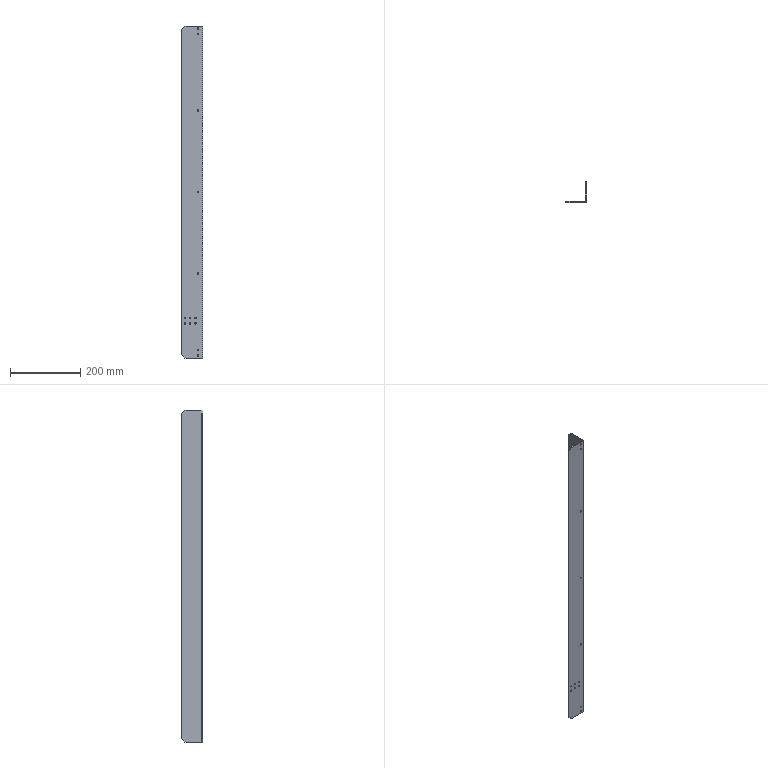Part | SolidWorks | features HoleWzd 2, Chamfer 1, Extrusion 1 | 1 solid | 38 faces | box 60 x 60 x 945 mm | volume 330466 mm3 | cylinder 26 | plane 12 | commonest cylinder face diameters 4.8 x14 4.2 x12
STEP:
#1=CARTESIAN_POINT('',(9.75,0.,-375.8));
#2=VERTEX_POINT('',#1);
#3=CARTESIAN_POINT('',(9.75,0.,-371.6));
#4=VERTEX_POINT('',#3);
#5=CARTESIAN_POINT('',(9.75,0.,-373.7));
#6=DIRECTION('',(0.,1.,0.));
#7=DIRECTION('',(0.,0.,1.));
#8=AXIS2_PLACEMENT_3D('',#5,#6,#7);
#9=CIRCLE('',#8,2.1);
#10=EDGE_CURVE('',#2,#4,#9,.T.);
#11=ORIENTED_EDGE('',*,*,#10,.F.);
#12=CARTESIAN_POINT('',(9.75,3.,-375.8));
#13=VERTEX_POINT('',#12);
#14=CARTESIAN_POINT('',(9.75,3.,-375.8));
#15=DIRECTION('',(0.,1.,0.));
#16=VECTOR('',#15,1000.);
#17=LINE('',#14,#16);
#18=EDGE_CURVE('',#2,#13,#17,.T.);
#19=ORIENTED_EDGE('',*,*,#18,.T.);
#20=CARTESIAN_POINT('',(9.75,3.,-371.6));
#21=VERTEX_POINT('',#20);
#22=CARTESIAN_POINT('',(9.75,3.,-373.7));
#23=DIRECTION('',(0.,1.,0.));
#24=DIRECTION('',(0.,0.,1.));
#25=AXIS2_PLACEMENT_3D('',#22,#23,#24);
#26=CIRCLE('',#25,2.1);
#27=EDGE_CURVE('',#13,#21,#26,.T.);
#28=ORIENTED_EDGE('',*,*,#27,.T.);
#29=CARTESIAN_POINT('',(9.75,3.,-371.6));
#30=DIRECTION('',(0.,1.,0.));
#31=VECTOR('',#30,1000.);
#32=LINE('',#29,#31);
#33=EDGE_CURVE('',#4,#21,#32,.T.);
#34=ORIENTED_EDGE('',*,*,#33,.F.);
#35=EDGE_LOOP('',(#11,#19,#28,#34));
#36=FACE_OUTER_BOUND('',#35,.T.);
#37=CARTESIAN_POINT('',(9.75,3.,-373.7));
#38=DIRECTION('',(0.,1.,0.));
#39=DIRECTION('',(0.,0.,1.));
#40=AXIS2_PLACEMENT_3D('',#37,#38,#39);
#41=CYLINDRICAL_SURFACE('',#40,2.1);
#42=ADVANCED_FACE('',(#36),#41,.F.);
#43=CARTESIAN_POINT('',(39.75,0.,-375.8));
#44=VERTEX_POINT('',#43);
#45=CARTESIAN_POINT('',(39.75,0.,-371.6));
#46=VERTEX_POINT('',#45);
#47=CARTESIAN_POINT('',(39.75,0.,-373.7));
#48=DIRECTION('',(0.,1.,0.));
#49=DIRECTION('',(0.,0.,1.));
#50=AXIS2_PLACEMENT_3D('',#47,#48,#49);
#51=CIRCLE('',#50,2.1);
#52=EDGE_CURVE('',#44,#46,#51,.T.);
#53=ORIENTED_EDGE('',*,*,#52,.F.);
#54=CARTESIAN_POINT('',(39.75,3.,-375.8));
#55=VERTEX_POINT('',#54);
#56=CARTESIAN_POINT('',(39.75,3.,-375.8));
#57=DIRECTION('',(0.,1.,0.));
#58=VECTOR('',#57,1000.);
#59=LINE('',#56,#58);
#60=EDGE_CURVE('',#44,#55,#59,.T.);
#61=ORIENTED_EDGE('',*,*,#60,.T.);
#62=CARTESIAN_POINT('',(39.75,3.,-371.6));
#63=VERTEX_POINT('',#62);
#64=CARTESIAN_POINT('',(39.75,3.,-373.7));
#65=DIRECTION('',(0.,1.,0.));
#66=DIRECTION('',(0.,0.,1.));
#67=AXIS2_PLACEMENT_3D('',#64,#65,#66);
#68=CIRCLE('',#67,2.1);
#69=EDGE_CURVE('',#55,#63,#68,.T.);
#70=ORIENTED_EDGE('',*,*,#69,.T.);
#71=CARTESIAN_POINT('',(39.75,3.,-371.6));
#72=DIRECTION('',(0.,1.,0.));
#73=VECTOR('',#72,1000.);
#74=LINE('',#71,#73);
#75=EDGE_CURVE('',#46,#63,#74,.T.);
#76=ORIENTED_EDGE('',*,*,#75,.F.);
#77=EDGE_LOOP('',(#53,#61,#70,#76));
#78=FACE_OUTER_BOUND('',#77,.T.);
#79=CARTESIAN_POINT('',(39.75,3.,-373.7));
#80=DIRECTION('',(0.,1.,0.));
#81=DIRECTION('',(0.,0.,1.));
#82=AXIS2_PLACEMENT_3D('',#79,#80,#81);
#83=CYLINDRICAL_SURFACE('',#82,2.1);
#84=ADVANCED_FACE('',(#78),#83,.F.);
#85=CARTESIAN_POINT('',(24.75,0.,-360.8));
#86=VERTEX_POINT('',#85);
#87=CARTESIAN_POINT('',(24.75,0.,-356.6));
#88=VERTEX_POINT('',#87);
#89=CARTESIAN_POINT('',(24.75,0.,-358.7));
#90=DIRECTION('',(0.,1.,0.));
#91=DIRECTION('',(0.,0.,1.));
#92=AXIS2_PLACEMENT_3D('',#89,#90,#91);
#93=CIRCLE('',#92,2.1);
#94=EDGE_CURVE('',#86,#88,#93,.T.);
#95=ORIENTED_EDGE('',*,*,#94,.F.);
#96=CARTESIAN_POINT('',(24.75,3.,-360.8));
#97=VERTEX_POINT('',#96);
#98=CARTESIAN_POINT('',(24.75,3.,-360.8));
#99=DIRECTION('',(0.,1.,0.));
#100=VECTOR('',#99,1000.);
#101=LINE('',#98,#100);
#102=EDGE_CURVE('',#86,#97,#101,.T.);
#103=ORIENTED_EDGE('',*,*,#102,.T.);
#104=CARTESIAN_POINT('',(24.75,3.,-356.6));
#105=VERTEX_POINT('',#104);
#106=CARTESIAN_POINT('',(24.75,3.,-358.7));
#107=DIRECTION('',(0.,1.,0.));
#108=DIRECTION('',(0.,0.,1.));
#109=AXIS2_PLACEMENT_3D('',#106,#107,#108);
#110=CIRCLE('',#109,2.1);
#111=EDGE_CURVE('',#97,#105,#110,.T.);
#112=ORIENTED_EDGE('',*,*,#111,.T.);
#113=CARTESIAN_POINT('',(24.75,3.,-356.6));
#114=DIRECTION('',(0.,1.,0.));
#115=VECTOR('',#114,1000.);
#116=LINE('',#113,#115);
#117=EDGE_CURVE('',#88,#105,#116,.T.);
#118=ORIENTED_EDGE('',*,*,#117,.F.);
#119=EDGE_LOOP('',(#95,#103,#112,#118));
#120=FACE_OUTER_BOUND('',#119,.T.);
#121=CARTESIAN_POINT('',(24.75,3.,-358.7));
#122=DIRECTION('',(0.,1.,0.));
#123=DIRECTION('',(0.,0.,1.));
#124=AXIS2_PLACEMENT_3D('',#121,#122,#123);
#125=CYLINDRICAL_SURFACE('',#124,2.1);
#126=ADVANCED_FACE('',(#120),#125,.F.);
#127=CARTESIAN_POINT('',(9.75,0.,-360.8));
#128=VERTEX_POINT('',#127);
#129=CARTESIAN_POINT('',(9.75,0.,-356.6));
#130=VERTEX_POINT('',#129);
#131=CARTESIAN_POINT('',(9.75,0.,-358.7));
#132=DIRECTION('',(0.,1.,0.));
#133=DIRECTION('',(0.,0.,1.));
#134=AXIS2_PLACEMENT_3D('',#131,#132,#133);
#135=CIRCLE('',#134,2.1);
#136=EDGE_CURVE('',#128,#130,#135,.T.);
#137=ORIENTED_EDGE('',*,*,#136,.F.);
#138=CARTESIAN_POINT('',(9.75,3.,-360.8));
#139=VERTEX_POINT('',#138);
#140=CARTESIAN_POINT('',(9.75,3.,-360.8));
#141=DIRECTION('',(0.,1.,0.));
#142=VECTOR('',#141,1000.);
#143=LINE('',#140,#142);
#144=EDGE_CURVE('',#128,#139,#143,.T.);
#145=ORIENTED_EDGE('',*,*,#144,.T.);
#146=CARTESIAN_POINT('',(9.75,3.,-356.6));
#147=VERTEX_POINT('',#146);
#148=CARTESIAN_POINT('',(9.75,3.,-358.7));
#149=DIRECTION('',(0.,1.,0.));
#150=DIRECTION('',(0.,0.,1.));
#151=AXIS2_PLACEMENT_3D('',#148,#149,#150);
#152=CIRCLE('',#151,2.1);
#153=EDGE_CURVE('',#139,#147,#152,.T.);
#154=ORIENTED_EDGE('',*,*,#153,.T.);
#155=CARTESIAN_POINT('',(9.75,3.,-356.6));
#156=DIRECTION('',(0.,1.,0.));
#157=VECTOR('',#156,1000.);
#158=LINE('',#155,#157);
#159=EDGE_CURVE('',#130,#147,#158,.T.);
#160=ORIENTED_EDGE('',*,*,#159,.F.);
#161=EDGE_LOOP('',(#137,#145,#154,#160));
#162=FACE_OUTER_BOUND('',#161,.T.);
#163=CARTESIAN_POINT('',(9.75,3.,-358.7));
#164=DIRECTION('',(0.,1.,0.));
#165=DIRECTION('',(0.,0.,1.));
#166=AXIS2_PLACEMENT_3D('',#163,#164,#165);
#167=CYLINDRICAL_SURFACE('',#166,2.1);
#168=ADVANCED_FACE('',(#162),#167,.F.);
#169=CARTESIAN_POINT('',(39.75,0.,-360.8));
#170=VERTEX_POINT('',#169);
#171=CARTESIAN_POINT('',(39.75,0.,-356.6));
#172=VERTEX_POINT('',#171);
#173=CARTESIAN_POINT('',(39.75,0.,-358.7));
#174=DIRECTION('',(0.,1.,0.));
#175=DIRECTION('',(0.,0.,1.));
#176=AXIS2_PLACEMENT_3D('',#173,#174,#175);
#177=CIRCLE('',#176,2.1);
#178=EDGE_CURVE('',#170,#172,#177,.T.);
#179=ORIENTED_EDGE('',*,*,#178,.F.);
#180=CARTESIAN_POINT('',(39.75,3.,-360.8));
#181=VERTEX_POINT('',#180);
#182=CARTESIAN_POINT('',(39.75,3.,-360.8));
#183=DIRECTION('',(0.,1.,0.));
#184=VECTOR('',#183,1000.);
#185=LINE('',#182,#184);
#186=EDGE_CURVE('',#170,#181,#185,.T.);
#187=ORIENTED_EDGE('',*,*,#186,.T.);
#188=CARTESIAN_POINT('',(39.75,3.,-356.6));
#189=VERTEX_POINT('',#188);
#190=CARTESIAN_POINT('',(39.75,3.,-358.7));
#191=DIRECTION('',(0.,1.,0.));
#192=DIRECTION('',(0.,0.,1.));
#193=AXIS2_PLACEMENT_3D('',#190,#191,#192);
#194=CIRCLE('',#193,2.1);
#195=EDGE_CURVE('',#181,#189,#194,.T.);
#196=ORIENTED_EDGE('',*,*,#195,.T.);
#197=CARTESIAN_POINT('',(39.75,3.,-356.6));
#198=DIRECTION('',(0.,1.,0.));
#199=VECTOR('',#198,1000.);
#200=LINE('',#197,#199);
#201=EDGE_CURVE('',#172,#189,#200,.T.);
#202=ORIENTED_EDGE('',*,*,#201,.F.);
#203=EDGE_LOOP('',(#179,#187,#196,#202));
#204=FACE_OUTER_BOUND('',#203,.T.);
#205=CARTESIAN_POINT('',(39.75,3.,-358.7));
#206=DIRECTION('',(0.,1.,0.));
#207=DIRECTION('',(0.,0.,1.));
#208=AXIS2_PLACEMENT_3D('',#205,#206,#207);
#209=CYLINDRICAL_SURFACE('',#208,2.1);
#210=ADVANCED_FACE('',(#204),#209,.F.);
#211=CARTESIAN_POINT('',(24.75,0.,-375.8));
#212=VERTEX_POINT('',#211);
#213=CARTESIAN_POINT('',(24.75,0.,-371.6));
#214=VERTEX_POINT('',#213);
#215=CARTESIAN_POINT('',(24.75,0.,-373.7));
#216=DIRECTION('',(0.,1.,0.));
#217=DIRECTION('',(0.,0.,1.));
#218=AXIS2_PLACEMENT_3D('',#215,#216,#217);
#219=CIRCLE('',#218,2.1);
#220=EDGE_CURVE('',#212,#214,#219,.T.);
#221=ORIENTED_EDGE('',*,*,#220,.F.);
#222=CARTESIAN_POINT('',(24.75,3.,-375.8));
#223=VERTEX_POINT('',#222);
#224=CARTESIAN_POINT('',(24.75,3.,-375.8));
#225=DIRECTION('',(0.,1.,0.));
#226=VECTOR('',#225,1000.);
#227=LINE('',#224,#226);
#228=EDGE_CURVE('',#212,#223,#227,.T.);
#229=ORIENTED_EDGE('',*,*,#228,.T.);
#230=CARTESIAN_POINT('',(24.75,3.,-371.6));
#231=VERTEX_POINT('',#230);
#232=CARTESIAN_POINT('',(24.75,3.,-373.7));
#233=DIRECTION('',(0.,1.,0.));
#234=DIRECTION('',(0.,0.,1.));
#235=AXIS2_PLACEMENT_3D('',#232,#233,#234);
#236=CIRCLE('',#235,2.1);
#237=EDGE_CURVE('',#223,#231,#236,.T.);
#238=ORIENTED_EDGE('',*,*,#237,.T.);
#239=CARTESIAN_POINT('',(24.75,3.,-371.6));
#240=DIRECTION('',(0.,1.,0.));
#241=VECTOR('',#240,1000.);
#242=LINE('',#239,#241);
#243=EDGE_CURVE('',#214,#231,#242,.T.);
#244=ORIENTED_EDGE('',*,*,#243,.F.);
#245=EDGE_LOOP('',(#221,#229,#238,#244));
#246=FACE_OUTER_BOUND('',#245,.T.);
#247=CARTESIAN_POINT('',(24.75,3.,-373.7));
#248=DIRECTION('',(0.,1.,0.));
#249=DIRECTION('',(0.,0.,1.));
#250=AXIS2_PLACEMENT_3D('',#247,#248,#249);
#251=CYLINDRICAL_SURFACE('',#250,2.1);
#252=ADVANCED_FACE('',(#246),#251,.F.);
#253=CARTESIAN_POINT('',(47.,0.,-2.4));
#254=VERTEX_POINT('',#253);
#255=CARTESIAN_POINT('',(47.,0.,2.4));
#256=VERTEX_POINT('',#255);
#257=CARTESIAN_POINT('',(47.,0.,0.));
#258=DIRECTION('',(0.,1.,0.));
#259=DIRECTION('',(0.,0.,1.));
#260=AXIS2_PLACEMENT_3D('',#257,#258,#259);
#261=CIRCLE('',#260,2.4);
#262=EDGE_CURVE('',#254,#256,#261,.T.);
#263=ORIENTED_EDGE('',*,*,#262,.F.);
#264=CARTESIAN_POINT('',(47.,3.,-2.4));
#265=VERTEX_POINT('',#264);
#266=CARTESIAN_POINT('',(47.,3.,-2.4));
#267=DIRECTION('',(0.,1.,0.));
#268=VECTOR('',#267,1000.);
#269=LINE('',#266,#268);
#270=EDGE_CURVE('',#254,#265,#269,.T.);
#271=ORIENTED_EDGE('',*,*,#270,.T.);
#272=CARTESIAN_POINT('',(47.,3.,2.4));
#273=VERTEX_POINT('',#272);
#274=CARTESIAN_POINT('',(47.,3.,0.));
#275=DIRECTION('',(0.,1.,0.));
#276=DIRECTION('',(0.,0.,1.));
#277=AXIS2_PLACEMENT_3D('',#274,#275,#276);
#278=CIRCLE('',#277,2.4);
#279=EDGE_CURVE('',#265,#273,#278,.T.);
#280=ORIENTED_EDGE('',*,*,#279,.T.);
#281=CARTESIAN_POINT('',(47.,3.,2.4));
#282=DIRECTION('',(0.,1.,0.));
#283=VECTOR('',#282,1000.);
#284=LINE('',#281,#283);
#285=EDGE_CURVE('',#256,#273,#284,.T.);
#286=ORIENTED_EDGE('',*,*,#285,.F.);
#287=EDGE_LOOP('',(#263,#271,#280,#286));
#288=FACE_OUTER_BOUND('',#287,.T.);
#289=CARTESIAN_POINT('',(47.,3.,0.));
#290=DIRECTION('',(0.,1.,0.));
#291=DIRECTION('',(0.,0.,1.));
#292=AXIS2_PLACEMENT_3D('',#289,#290,#291);
#293=CYLINDRICAL_SURFACE('',#292,2.4);
#294=ADVANCED_FACE('',(#288),#293,.F.);
#295=CARTESIAN_POINT('',(47.,0.,-234.65));
#296=VERTEX_POINT('',#295);
#297=CARTESIAN_POINT('',(47.,0.,-229.85));
#298=VERTEX_POINT('',#297);
#299=CARTESIAN_POINT('',(47.,0.,-232.25));
#300=DIRECTION('',(0.,1.,0.));
#301=DIRECTION('',(0.,0.,1.));
#302=AXIS2_PLACEMENT_3D('',#299,#300,#301);
#303=CIRCLE('',#302,2.4);
#304=EDGE_CURVE('',#296,#298,#303,.T.);
#305=ORIENTED_EDGE('',*,*,#304,.F.);
#306=CARTESIAN_POINT('',(47.,3.,-234.65));
#307=VERTEX_POINT('',#306);
#308=CARTESIAN_POINT('',(47.,3.,-234.65));
#309=DIRECTION('',(0.,1.,0.));
#310=VECTOR('',#309,1000.);
#311=LINE('',#308,#310);
#312=EDGE_CURVE('',#296,#307,#311,.T.);
#313=ORIENTED_EDGE('',*,*,#312,.T.);
#314=CARTESIAN_POINT('',(47.,3.,-229.85));
#315=VERTEX_POINT('',#314);
#316=CARTESIAN_POINT('',(47.,3.,-232.25));
#317=DIRECTION('',(0.,1.,0.));
#318=DIRECTION('',(0.,0.,1.));
#319=AXIS2_PLACEMENT_3D('',#316,#317,#318);
#320=CIRCLE('',#319,2.4);
#321=EDGE_CURVE('',#307,#315,#320,.T.);
#322=ORIENTED_EDGE('',*,*,#321,.T.);
#323=CARTESIAN_POINT('',(47.,3.,-229.85));
#324=DIRECTION('',(0.,1.,0.));
#325=VECTOR('',#324,1000.);
#326=LINE('',#323,#325);
#327=EDGE_CURVE('',#298,#315,#326,.T.);
#328=ORIENTED_EDGE('',*,*,#327,.F.);
#329=EDGE_LOOP('',(#305,#313,#322,#328));
#330=FACE_OUTER_BOUND('',#329,.T.);
#331=CARTESIAN_POINT('',(47.,3.,-232.25));
#332=DIRECTION('',(0.,1.,0.));
#333=DIRECTION('',(0.,0.,1.));
#334=AXIS2_PLACEMENT_3D('',#331,#332,#333);
#335=CYLINDRICAL_SURFACE('',#334,2.4);
#336=ADVANCED_FACE('',(#330),#335,.F.);
#337=CARTESIAN_POINT('',(47.,0.,-466.9));
#338=VERTEX_POINT('',#337);
#339=CARTESIAN_POINT('',(47.,0.,-462.1));
#340=VERTEX_POINT('',#339);
#341=CARTESIAN_POINT('',(47.,0.,-464.5));
#342=DIRECTION('',(0.,1.,0.));
#343=DIRECTION('',(0.,0.,1.));
#344=AXIS2_PLACEMENT_3D('',#341,#342,#343);
#345=CIRCLE('',#344,2.4);
#346=EDGE_CURVE('',#338,#340,#345,.T.);
#347=ORIENTED_EDGE('',*,*,#346,.F.);
#348=CARTESIAN_POINT('',(47.,3.,-466.9));
#349=VERTEX_POINT('',#348);
#350=CARTESIAN_POINT('',(47.,3.,-466.9));
#351=DIRECTION('',(0.,1.,0.));
#352=VECTOR('',#351,1000.);
#353=LINE('',#350,#352);
#354=EDGE_CURVE('',#338,#349,#353,.T.);
#355=ORIENTED_EDGE('',*,*,#354,.T.);
#356=CARTESIAN_POINT('',(47.,3.,-462.1));
#357=VERTEX_POINT('',#356);
#358=CARTESIAN_POINT('',(47.,3.,-464.5));
#359=DIRECTION('',(0.,1.,0.));
#360=DIRECTION('',(0.,0.,1.));
#361=AXIS2_PLACEMENT_3D('',#358,#359,#360);
#362=CIRCLE('',#361,2.4);
#363=EDGE_CURVE('',#349,#357,#362,.T.);
#364=ORIENTED_EDGE('',*,*,#363,.T.);
#365=CARTESIAN_POINT('',(47.,3.,-462.1));
#366=DIRECTION('',(0.,1.,0.));
#367=VECTOR('',#366,1000.);
#368=LINE('',#365,#367);
#369=EDGE_CURVE('',#340,#357,#368,.T.);
#370=ORIENTED_EDGE('',*,*,#369,.F.);
#371=EDGE_LOOP('',(#347,#355,#364,#370));
#372=FACE_OUTER_BOUND('',#371,.T.);
#373=CARTESIAN_POINT('',(47.,3.,-464.5));
#374=DIRECTION('',(0.,1.,0.));
#375=DIRECTION('',(0.,0.,1.));
#376=AXIS2_PLACEMENT_3D('',#373,#374,#375);
#377=CYLINDRICAL_SURFACE('',#376,2.4);
#378=ADVANCED_FACE('',(#372),#377,.F.);
#379=CARTESIAN_POINT('',(47.,0.,462.1));
#380=VERTEX_POINT('',#379);
#381=CARTESIAN_POINT('',(47.,0.,466.9));
#382=VERTEX_POINT('',#381);
#383=CARTESIAN_POINT('',(47.,0.,464.5));
#384=DIRECTION('',(0.,1.,0.));
#385=DIRECTION('',(0.,0.,1.));
#386=AXIS2_PLACEMENT_3D('',#383,#384,#385);
#387=CIRCLE('',#386,2.4);
#388=EDGE_CURVE('',#380,#382,#387,.T.);
#389=ORIENTED_EDGE('',*,*,#388,.F.);
#390=CARTESIAN_POINT('',(47.,3.,462.1));
#391=VERTEX_POINT('',#390);
#392=CARTESIAN_POINT('',(47.,3.,462.1));
#393=DIRECTION('',(0.,1.,0.));
#394=VECTOR('',#393,1000.);
#395=LINE('',#392,#394);
#396=EDGE_CURVE('',#380,#391,#395,.T.);
#397=ORIENTED_EDGE('',*,*,#396,.T.);
#398=CARTESIAN_POINT('',(47.,3.,466.9));
#399=VERTEX_POINT('',#398);
#400=CARTESIAN_POINT('',(47.,3.,464.5));
#401=DIRECTION('',(0.,1.,0.));
#402=DIRECTION('',(0.,0.,1.));
#403=AXIS2_PLACEMENT_3D('',#400,#401,#402);
#404=CIRCLE('',#403,2.4);
#405=EDGE_CURVE('',#391,#399,#404,.T.);
#406=ORIENTED_EDGE('',*,*,#405,.T.);
#407=CARTESIAN_POINT('',(47.,3.,466.9));
#408=DIRECTION('',(0.,1.,0.));
#409=VECTOR('',#408,1000.);
#410=LINE('',#407,#409);
#411=EDGE_CURVE('',#382,#399,#410,.T.);
#412=ORIENTED_EDGE('',*,*,#411,.F.);
#413=EDGE_LOOP('',(#389,#397,#406,#412));
#414=FACE_OUTER_BOUND('',#413,.T.);
#415=CARTESIAN_POINT('',(47.,3.,464.5));
#416=DIRECTION('',(0.,1.,0.));
#417=DIRECTION('',(0.,0.,1.));
#418=AXIS2_PLACEMENT_3D('',#415,#416,#417);
#419=CYLINDRICAL_SURFACE('',#418,2.4);
#420=ADVANCED_FACE('',(#414),#419,.F.);
#421=CARTESIAN_POINT('',(47.,0.,229.85));
#422=VERTEX_POINT('',#421);
#423=CARTESIAN_POINT('',(47.,0.,234.65));
#424=VERTEX_POINT('',#423);
#425=CARTESIAN_POINT('',(47.,0.,232.25));
#426=DIRECTION('',(0.,1.,0.));
#427=DIRECTION('',(0.,0.,1.));
#428=AXIS2_PLACEMENT_3D('',#425,#426,#427);
#429=CIRCLE('',#428,2.4);
#430=EDGE_CURVE('',#422,#424,#429,.T.);
#431=ORIENTED_EDGE('',*,*,#430,.F.);
#432=CARTESIAN_POINT('',(47.,3.,229.85));
#433=VERTEX_POINT('',#432);
#434=CARTESIAN_POINT('',(47.,3.,229.85));
#435=DIRECTION('',(0.,1.,0.));
#436=VECTOR('',#435,1000.);
#437=LINE('',#434,#436);
#438=EDGE_CURVE('',#422,#433,#437,.T.);
#439=ORIENTED_EDGE('',*,*,#438,.T.);
#440=CARTESIAN_POINT('',(47.,3.,234.65));
#441=VERTEX_POINT('',#440);
#442=CARTESIAN_POINT('',(47.,3.,232.25));
#443=DIRECTION('',(0.,1.,0.));
#444=DIRECTION('',(0.,0.,1.));
#445=AXIS2_PLACEMENT_3D('',#442,#443,#444);
#446=CIRCLE('',#445,2.4);
#447=EDGE_CURVE('',#433,#441,#446,.T.);
#448=ORIENTED_EDGE('',*,*,#447,.T.);
#449=CARTESIAN_POINT('',(47.,3.,234.65));
#450=DIRECTION('',(0.,1.,0.));
#451=VECTOR('',#450,1000.);
#452=LINE('',#449,#451);
#453=EDGE_CURVE('',#424,#441,#452,.T.);
#454=ORIENTED_EDGE('',*,*,#453,.F.);
#455=EDGE_LOOP('',(#431,#439,#448,#454));
#456=FACE_OUTER_BOUND('',#455,.T.);
#457=CARTESIAN_POINT('',(47.,3.,232.25));
#458=DIRECTION('',(0.,1.,0.));
#459=DIRECTION('',(0.,0.,1.));
#460=AXIS2_PLACEMENT_3D('',#457,#458,#459);
#461=CYLINDRICAL_SURFACE('',#460,2.4);
#462=ADVANCED_FACE('',(#456),#461,.F.);
#463=CARTESIAN_POINT('',(47.,0.,-451.9));
#464=VERTEX_POINT('',#463);
#465=CARTESIAN_POINT('',(47.,0.,-447.1));
#466=VERTEX_POINT('',#465);
#467=CARTESIAN_POINT('',(47.,0.,-449.5));
#468=DIRECTION('',(0.,1.,0.));
#469=DIRECTION('',(0.,0.,1.));
#470=AXIS2_PLACEMENT_3D('',#467,#468,#469);
#471=CIRCLE('',#470,2.4);
#472=EDGE_CURVE('',#464,#466,#471,.T.);
#473=ORIENTED_EDGE('',*,*,#472,.F.);
#474=CARTESIAN_POINT('',(47.,3.,-451.9));
#475=VERTEX_POINT('',#474);
#476=CARTESIAN_POINT('',(47.,3.,-451.9));
#477=DIRECTION('',(0.,1.,0.));
#478=VECTOR('',#477,1000.);
#479=LINE('',#476,#478);
#480=EDGE_CURVE('',#464,#475,#479,.T.);
#481=ORIENTED_EDGE('',*,*,#480,.T.);
#482=CARTESIAN_POINT('',(47.,3.,-447.1));
#483=VERTEX_POINT('',#482);
#484=CARTESIAN_POINT('',(47.,3.,-449.5));
#485=DIRECTION('',(0.,1.,0.));
#486=DIRECTION('',(0.,0.,1.));
#487=AXIS2_PLACEMENT_3D('',#484,#485,#486);
#488=CIRCLE('',#487,2.4);
#489=EDGE_CURVE('',#475,#483,#488,.T.);
#490=ORIENTED_EDGE('',*,*,#489,.T.);
#491=CARTESIAN_POINT('',(47.,3.,-447.1));
#492=DIRECTION('',(0.,1.,0.));
#493=VECTOR('',#492,1000.);
#494=LINE('',#491,#493);
#495=EDGE_CURVE('',#466,#483,#494,.T.);
#496=ORIENTED_EDGE('',*,*,#495,.F.);
#497=EDGE_LOOP('',(#473,#481,#490,#496));
#498=FACE_OUTER_BOUND('',#497,.T.);
#499=CARTESIAN_POINT('',(47.,3.,-449.5));
#500=DIRECTION('',(0.,1.,0.));
#501=DIRECTION('',(0.,0.,1.));
#502=AXIS2_PLACEMENT_3D('',#499,#500,#501);
#503=CYLINDRICAL_SURFACE('',#502,2.4);
#504=ADVANCED_FACE('',(#498),#503,.F.);
#505=CARTESIAN_POINT('',(47.,0.,447.1));
#506=VERTEX_POINT('',#505);
#507=CARTESIAN_POINT('',(47.,0.,451.9));
#508=VERTEX_POINT('',#507);
#509=CARTESIAN_POINT('',(47.,0.,449.5));
#510=DIRECTION('',(0.,1.,0.));
#511=DIRECTION('',(0.,0.,1.));
#512=AXIS2_PLACEMENT_3D('',#509,#510,#511);
#513=CIRCLE('',#512,2.4);
#514=EDGE_CURVE('',#506,#508,#513,.T.);
#515=ORIENTED_EDGE('',*,*,#514,.F.);
#516=CARTESIAN_POINT('',(47.,3.,447.1));
#517=VERTEX_POINT('',#516);
#518=CARTESIAN_POINT('',(47.,3.,447.1));
#519=DIRECTION('',(0.,1.,0.));
#520=VECTOR('',#519,1000.);
#521=LINE('',#518,#520);
#522=EDGE_CURVE('',#506,#517,#521,.T.);
#523=ORIENTED_EDGE('',*,*,#522,.T.);
#524=CARTESIAN_POINT('',(47.,3.,451.9));
#525=VERTEX_POINT('',#524);
#526=CARTESIAN_POINT('',(47.,3.,449.5));
#527=DIRECTION('',(0.,1.,0.));
#528=DIRECTION('',(0.,0.,1.));
#529=AXIS2_PLACEMENT_3D('',#526,#527,#528);
#530=CIRCLE('',#529,2.4);
#531=EDGE_CURVE('',#517,#525,#530,.T.);
#532=ORIENTED_EDGE('',*,*,#531,.T.);
#533=CARTESIAN_POINT('',(47.,3.,451.9));
#534=DIRECTION('',(0.,1.,0.));
#535=VECTOR('',#534,1000.);
#536=LINE('',#533,#535);
#537=EDGE_CURVE('',#508,#525,#536,.T.);
#538=ORIENTED_EDGE('',*,*,#537,.F.);
#539=EDGE_LOOP('',(#515,#523,#532,#538));
#540=FACE_OUTER_BOUND('',#539,.T.);
#541=CARTESIAN_POINT('',(47.,3.,449.5));
#542=DIRECTION('',(0.,1.,0.));
#543=DIRECTION('',(0.,0.,1.));
#544=AXIS2_PLACEMENT_3D('',#541,#542,#543);
#545=CYLINDRICAL_SURFACE('',#544,2.4);
#546=ADVANCED_FACE('',(#540),#545,.F.);
#547=CARTESIAN_POINT('',(47.,3.,0.));
#548=DIRECTION('',(0.,1.,0.));
#549=DIRECTION('',(0.,0.,1.));
#550=AXIS2_PLACEMENT_3D('',#547,#548,#549);
#551=CIRCLE('',#550,2.4);
#552=EDGE_CURVE('',#273,#265,#551,.T.);
#553=ORIENTED_EDGE('',*,*,#552,.F.);
#554=ORIENTED_EDGE('',*,*,#279,.F.);
#555=EDGE_LOOP('',(#553,#554));
#556=FACE_BOUND('',#555,.T.);
#557=CARTESIAN_POINT('',(47.,3.,-232.25));
#558=DIRECTION('',(0.,1.,0.));
#559=DIRECTION('',(0.,0.,1.));
#560=AXIS2_PLACEMENT_3D('',#557,#558,#559);
#561=CIRCLE('',#560,2.4);
#562=EDGE_CURVE('',#315,#307,#561,.T.);
#563=ORIENTED_EDGE('',*,*,#562,.F.);
#564=ORIENTED_EDGE('',*,*,#321,.F.);
#565=EDGE_LOOP('',(#563,#564));
#566=FACE_BOUND('',#565,.T.);
#567=CARTESIAN_POINT('',(47.,3.,-464.5));
#568=DIRECTION('',(0.,1.,0.));
#569=DIRECTION('',(0.,0.,1.));
#570=AXIS2_PLACEMENT_3D('',#567,#568,#569);
#571=CIRCLE('',#570,2.4);
#572=EDGE_CURVE('',#357,#349,#571,.T.);
#573=ORIENTED_EDGE('',*,*,#572,.F.);
#574=ORIENTED_EDGE('',*,*,#363,.F.);
#575=EDGE_LOOP('',(#573,#574));
#576=FACE_BOUND('',#575,.T.);
#577=CARTESIAN_POINT('',(47.,3.,464.5));
#578=DIRECTION('',(0.,1.,0.));
#579=DIRECTION('',(0.,0.,1.));
#580=AXIS2_PLACEMENT_3D('',#577,#578,#579);
#581=CIRCLE('',#580,2.4);
#582=EDGE_CURVE('',#399,#391,#581,.T.);
#583=ORIENTED_EDGE('',*,*,#582,.F.);
#584=ORIENTED_EDGE('',*,*,#405,.F.);
#585=EDGE_LOOP('',(#583,#584));
#586=FACE_BOUND('',#585,.T.);
#587=CARTESIAN_POINT('',(47.,3.,232.25));
#588=DIRECTION('',(0.,1.,0.));
#589=DIRECTION('',(0.,0.,1.));
#590=AXIS2_PLACEMENT_3D('',#587,#588,#589);
#591=CIRCLE('',#590,2.4);
#592=EDGE_CURVE('',#441,#433,#591,.T.);
#593=ORIENTED_EDGE('',*,*,#592,.F.);
#594=ORIENTED_EDGE('',*,*,#447,.F.);
#595=EDGE_LOOP('',(#593,#594));
#596=FACE_BOUND('',#595,.T.);
#597=CARTESIAN_POINT('',(47.,3.,-449.5));
#598=DIRECTION('',(0.,1.,0.));
#599=DIRECTION('',(0.,0.,1.));
#600=AXIS2_PLACEMENT_3D('',#597,#598,#599);
#601=CIRCLE('',#600,2.4);
#602=EDGE_CURVE('',#483,#475,#601,.T.);
#603=ORIENTED_EDGE('',*,*,#602,.F.);
#604=ORIENTED_EDGE('',*,*,#489,.F.);
#605=EDGE_LOOP('',(#603,#604));
#606=FACE_BOUND('',#605,.T.);
#607=CARTESIAN_POINT('',(47.,3.,449.5));
#608=DIRECTION('',(0.,1.,0.));
#609=DIRECTION('',(0.,0.,1.));
#610=AXIS2_PLACEMENT_3D('',#607,#608,#609);
#611=CIRCLE('',#610,2.4);
#612=EDGE_CURVE('',#525,#517,#611,.T.);
#613=ORIENTED_EDGE('',*,*,#612,.F.);
#614=ORIENTED_EDGE('',*,*,#531,.F.);
#615=EDGE_LOOP('',(#613,#614));
#616=FACE_BOUND('',#615,.T.);
#617=CARTESIAN_POINT('',(57.,3.,-472.5));
#618=VERTEX_POINT('',#617);
#619=CARTESIAN_POINT('',(10.,3.,-472.5));
#620=VERTEX_POINT('',#619);
#621=CARTESIAN_POINT('',(57.,3.,-472.5));
#622=DIRECTION('',(-1.,0.,0.));
#623=VECTOR('',#622,1000.);
#624=LINE('',#621,#623);
#625=EDGE_CURVE('',#618,#620,#624,.T.);
#626=ORIENTED_EDGE('',*,*,#625,.T.);
#627=CARTESIAN_POINT('',(0.,3.,-462.5));
#628=VERTEX_POINT('',#627);
#629=CARTESIAN_POINT('',(0.,3.,-462.5));
#630=DIRECTION('',(-0.7071,0.,0.7071));
#631=VECTOR('',#630,1000.);
#632=LINE('',#629,#631);
#633=EDGE_CURVE('',#620,#628,#632,.T.);
#634=ORIENTED_EDGE('',*,*,#633,.T.);
#635=CARTESIAN_POINT('',(0.,3.,462.5));
#636=VERTEX_POINT('',#635);
#637=CARTESIAN_POINT('',(0.,3.,472.5));
#638=DIRECTION('',(0.,0.,-1.));
#639=VECTOR('',#638,1000.);
#640=LINE('',#637,#639);
#641=EDGE_CURVE('',#636,#628,#640,.T.);
#642=ORIENTED_EDGE('',*,*,#641,.F.);
#643=CARTESIAN_POINT('',(10.,3.,472.5));
#644=VERTEX_POINT('',#643);
#645=CARTESIAN_POINT('',(10.,3.,472.5));
#646=DIRECTION('',(0.7071,0.,0.7071));
#647=VECTOR('',#646,1000.);
#648=LINE('',#645,#647);
#649=EDGE_CURVE('',#636,#644,#648,.T.);
#650=ORIENTED_EDGE('',*,*,#649,.T.);
#651=CARTESIAN_POINT('',(57.,3.,472.5));
#652=VERTEX_POINT('',#651);
#653=CARTESIAN_POINT('',(57.,3.,472.5));
#654=DIRECTION('',(-1.,0.,0.));
#655=VECTOR('',#654,1000.);
#656=LINE('',#653,#655);
#657=EDGE_CURVE('',#652,#644,#656,.T.);
#658=ORIENTED_EDGE('',*,*,#657,.F.);
#659=CARTESIAN_POINT('',(57.,3.,472.5));
#660=DIRECTION('',(0.,0.,-1.));
#661=VECTOR('',#660,1000.);
#662=LINE('',#659,#661);
#663=EDGE_CURVE('',#652,#618,#662,.T.);
#664=ORIENTED_EDGE('',*,*,#663,.T.);
#665=EDGE_LOOP('',(#626,#634,#642,#650,#658,#664));
#666=FACE_OUTER_BOUND('',#665,.T.);
#667=CARTESIAN_POINT('',(24.75,3.,-373.7));
#668=DIRECTION('',(0.,1.,0.));
#669=DIRECTION('',(0.,0.,1.));
#670=AXIS2_PLACEMENT_3D('',#667,#668,#669);
#671=CIRCLE('',#670,2.1);
#672=EDGE_CURVE('',#231,#223,#671,.T.);
#673=ORIENTED_EDGE('',*,*,#672,.F.);
#674=ORIENTED_EDGE('',*,*,#237,.F.);
#675=EDGE_LOOP('',(#673,#674));
#676=FACE_BOUND('',#675,.T.);
#677=CARTESIAN_POINT('',(39.75,3.,-358.7));
#678=DIRECTION('',(0.,1.,0.));
#679=DIRECTION('',(0.,0.,1.));
#680=AXIS2_PLACEMENT_3D('',#677,#678,#679);
#681=CIRCLE('',#680,2.1);
#682=EDGE_CURVE('',#189,#181,#681,.T.);
#683=ORIENTED_EDGE('',*,*,#682,.F.);
#684=ORIENTED_EDGE('',*,*,#195,.F.);
#685=EDGE_LOOP('',(#683,#684));
#686=FACE_BOUND('',#685,.T.);
#687=CARTESIAN_POINT('',(9.75,3.,-358.7));
#688=DIRECTION('',(0.,1.,0.));
#689=DIRECTION('',(0.,0.,1.));
#690=AXIS2_PLACEMENT_3D('',#687,#688,#689);
#691=CIRCLE('',#690,2.1);
#692=EDGE_CURVE('',#147,#139,#691,.T.);
#693=ORIENTED_EDGE('',*,*,#692,.F.);
#694=ORIENTED_EDGE('',*,*,#153,.F.);
#695=EDGE_LOOP('',(#693,#694));
#696=FACE_BOUND('',#695,.T.);
#697=CARTESIAN_POINT('',(24.75,3.,-358.7));
#698=DIRECTION('',(0.,1.,0.));
#699=DIRECTION('',(0.,0.,1.));
#700=AXIS2_PLACEMENT_3D('',#697,#698,#699);
#701=CIRCLE('',#700,2.1);
#702=EDGE_CURVE('',#105,#97,#701,.T.);
#703=ORIENTED_EDGE('',*,*,#702,.F.);
#704=ORIENTED_EDGE('',*,*,#111,.F.);
#705=EDGE_LOOP('',(#703,#704));
#706=FACE_BOUND('',#705,.T.);
#707=CARTESIAN_POINT('',(39.75,3.,-373.7));
#708=DIRECTION('',(0.,1.,0.));
#709=DIRECTION('',(0.,0.,1.));
#710=AXIS2_PLACEMENT_3D('',#707,#708,#709);
#711=CIRCLE('',#710,2.1);
#712=EDGE_CURVE('',#63,#55,#711,.T.);
#713=ORIENTED_EDGE('',*,*,#712,.F.);
#714=ORIENTED_EDGE('',*,*,#69,.F.);
#715=EDGE_LOOP('',(#713,#714));
#716=FACE_BOUND('',#715,.T.);
#717=CARTESIAN_POINT('',(9.75,3.,-373.7));
#718=DIRECTION('',(0.,1.,0.));
#719=DIRECTION('',(0.,0.,1.));
#720=AXIS2_PLACEMENT_3D('',#717,#718,#719);
#721=CIRCLE('',#720,2.1);
#722=EDGE_CURVE('',#21,#13,#721,.T.);
#723=ORIENTED_EDGE('',*,*,#722,.F.);
#724=ORIENTED_EDGE('',*,*,#27,.F.);
#725=EDGE_LOOP('',(#723,#724));
#726=FACE_BOUND('',#725,.T.);
#727=CARTESIAN_POINT('',(57.,3.,472.5));
#728=DIRECTION('',(0.,-1.,0.));
#729=DIRECTION('',(1.,0.,0.));
#730=AXIS2_PLACEMENT_3D('',#727,#728,#729);
#731=PLANE('',#730);
#732=ADVANCED_FACE('',(#556,#566,#576,#586,#596,#606,#616,#666,#676,#686,#696,#706,#716,#726),#731,.F.);
#733=ORIENTED_EDGE('',*,*,#641,.T.);
#734=CARTESIAN_POINT('',(0.,0.,-462.5));
#735=VERTEX_POINT('',#734);
#736=CARTESIAN_POINT('',(0.,3.,-462.5));
#737=DIRECTION('',(0.,-1.,0.));
#738=VECTOR('',#737,1000.);
#739=LINE('',#736,#738);
#740=EDGE_CURVE('',#628,#735,#739,.T.);
#741=ORIENTED_EDGE('',*,*,#740,.T.);
#742=CARTESIAN_POINT('',(0.,0.,462.5));
#743=VERTEX_POINT('',#742);
#744=CARTESIAN_POINT('',(0.,0.,472.5));
#745=DIRECTION('',(0.,0.,-1.));
#746=VECTOR('',#745,1000.);
#747=LINE('',#744,#746);
#748=EDGE_CURVE('',#743,#735,#747,.T.);
#749=ORIENTED_EDGE('',*,*,#748,.F.);
#750=CARTESIAN_POINT('',(0.,3.,462.5));
#751=DIRECTION('',(0.,1.,0.));
#752=VECTOR('',#751,1000.);
#753=LINE('',#750,#752);
#754=EDGE_CURVE('',#743,#636,#753,.T.);
#755=ORIENTED_EDGE('',*,*,#754,.T.);
#756=EDGE_LOOP('',(#733,#741,#749,#755));
#757=FACE_OUTER_BOUND('',#756,.T.);
#758=CARTESIAN_POINT('',(0.,3.,472.5));
#759=DIRECTION('',(1.,0.,0.));
#760=DIRECTION('',(0.,1.,0.));
#761=AXIS2_PLACEMENT_3D('',#758,#759,#760);
#762=PLANE('',#761);
#763=ADVANCED_FACE('',(#757),#762,.F.);
#764=CARTESIAN_POINT('',(9.75,0.,-373.7));
#765=DIRECTION('',(0.,1.,0.));
#766=DIRECTION('',(0.,0.,1.));
#767=AXIS2_PLACEMENT_3D('',#764,#765,#766);
#768=CIRCLE('',#767,2.1);
#769=EDGE_CURVE('',#4,#2,#768,.T.);
#770=ORIENTED_EDGE('',*,*,#769,.T.);
#771=ORIENTED_EDGE('',*,*,#10,.T.);
#772=EDGE_LOOP('',(#770,#771));
#773=FACE_BOUND('',#772,.T.);
#774=CARTESIAN_POINT('',(39.75,0.,-373.7));
#775=DIRECTION('',(0.,1.,0.));
#776=DIRECTION('',(0.,0.,1.));
#777=AXIS2_PLACEMENT_3D('',#774,#775,#776);
#778=CIRCLE('',#777,2.1);
#779=EDGE_CURVE('',#46,#44,#778,.T.);
#780=ORIENTED_EDGE('',*,*,#779,.T.);
#781=ORIENTED_EDGE('',*,*,#52,.T.);
#782=EDGE_LOOP('',(#780,#781));
#783=FACE_BOUND('',#782,.T.);
#784=CARTESIAN_POINT('',(24.75,0.,-358.7));
#785=DIRECTION('',(0.,1.,0.));
#786=DIRECTION('',(0.,0.,1.));
#787=AXIS2_PLACEMENT_3D('',#784,#785,#786);
#788=CIRCLE('',#787,2.1);
#789=EDGE_CURVE('',#88,#86,#788,.T.);
#790=ORIENTED_EDGE('',*,*,#789,.T.);
#791=ORIENTED_EDGE('',*,*,#94,.T.);
#792=EDGE_LOOP('',(#790,#791));
#793=FACE_BOUND('',#792,.T.);
#794=CARTESIAN_POINT('',(9.75,0.,-358.7));
#795=DIRECTION('',(0.,1.,0.));
#796=DIRECTION('',(0.,0.,1.));
#797=AXIS2_PLACEMENT_3D('',#794,#795,#796);
#798=CIRCLE('',#797,2.1);
#799=EDGE_CURVE('',#130,#128,#798,.T.);
#800=ORIENTED_EDGE('',*,*,#799,.T.);
#801=ORIENTED_EDGE('',*,*,#136,.T.);
#802=EDGE_LOOP('',(#800,#801));
#803=FACE_BOUND('',#802,.T.);
#804=CARTESIAN_POINT('',(39.75,0.,-358.7));
#805=DIRECTION('',(0.,1.,0.));
#806=DIRECTION('',(0.,0.,1.));
#807=AXIS2_PLACEMENT_3D('',#804,#805,#806);
#808=CIRCLE('',#807,2.1);
#809=EDGE_CURVE('',#172,#170,#808,.T.);
#810=ORIENTED_EDGE('',*,*,#809,.T.);
#811=ORIENTED_EDGE('',*,*,#178,.T.);
#812=EDGE_LOOP('',(#810,#811));
#813=FACE_BOUND('',#812,.T.);
#814=CARTESIAN_POINT('',(24.75,0.,-373.7));
#815=DIRECTION('',(0.,1.,0.));
#816=DIRECTION('',(0.,0.,1.));
#817=AXIS2_PLACEMENT_3D('',#814,#815,#816);
#818=CIRCLE('',#817,2.1);
#819=EDGE_CURVE('',#214,#212,#818,.T.);
#820=ORIENTED_EDGE('',*,*,#819,.T.);
#821=ORIENTED_EDGE('',*,*,#220,.T.);
#822=EDGE_LOOP('',(#820,#821));
#823=FACE_BOUND('',#822,.T.);
#824=CARTESIAN_POINT('',(47.,0.,0.));
#825=DIRECTION('',(0.,1.,0.));
#826=DIRECTION('',(0.,0.,1.));
#827=AXIS2_PLACEMENT_3D('',#824,#825,#826);
#828=CIRCLE('',#827,2.4);
#829=EDGE_CURVE('',#256,#254,#828,.T.);
#830=ORIENTED_EDGE('',*,*,#829,.T.);
#831=ORIENTED_EDGE('',*,*,#262,.T.);
#832=EDGE_LOOP('',(#830,#831));
#833=FACE_BOUND('',#832,.T.);
#834=CARTESIAN_POINT('',(47.,0.,-232.25));
#835=DIRECTION('',(0.,1.,0.));
#836=DIRECTION('',(0.,0.,1.));
#837=AXIS2_PLACEMENT_3D('',#834,#835,#836);
#838=CIRCLE('',#837,2.4);
#839=EDGE_CURVE('',#298,#296,#838,.T.);
#840=ORIENTED_EDGE('',*,*,#839,.T.);
#841=ORIENTED_EDGE('',*,*,#304,.T.);
#842=EDGE_LOOP('',(#840,#841));
#843=FACE_BOUND('',#842,.T.);
#844=CARTESIAN_POINT('',(47.,0.,-464.5));
#845=DIRECTION('',(0.,1.,0.));
#846=DIRECTION('',(0.,0.,1.));
#847=AXIS2_PLACEMENT_3D('',#844,#845,#846);
#848=CIRCLE('',#847,2.4);
#849=EDGE_CURVE('',#340,#338,#848,.T.);
#850=ORIENTED_EDGE('',*,*,#849,.T.);
#851=ORIENTED_EDGE('',*,*,#346,.T.);
#852=EDGE_LOOP('',(#850,#851));
#853=FACE_BOUND('',#852,.T.);
#854=CARTESIAN_POINT('',(47.,0.,464.5));
#855=DIRECTION('',(0.,1.,0.));
#856=DIRECTION('',(0.,0.,1.));
#857=AXIS2_PLACEMENT_3D('',#854,#855,#856);
#858=CIRCLE('',#857,2.4);
#859=EDGE_CURVE('',#382,#380,#858,.T.);
#860=ORIENTED_EDGE('',*,*,#859,.T.);
#861=ORIENTED_EDGE('',*,*,#388,.T.);
#862=EDGE_LOOP('',(#860,#861));
#863=FACE_BOUND('',#862,.T.);
#864=CARTESIAN_POINT('',(47.,0.,232.25));
#865=DIRECTION('',(0.,1.,0.));
#866=DIRECTION('',(0.,0.,1.));
#867=AXIS2_PLACEMENT_3D('',#864,#865,#866);
#868=CIRCLE('',#867,2.4);
#869=EDGE_CURVE('',#424,#422,#868,.T.);
#870=ORIENTED_EDGE('',*,*,#869,.T.);
#871=ORIENTED_EDGE('',*,*,#430,.T.);
#872=EDGE_LOOP('',(#870,#871));
#873=FACE_BOUND('',#872,.T.);
#874=CARTESIAN_POINT('',(47.,0.,-449.5));
#875=DIRECTION('',(0.,1.,0.));
#876=DIRECTION('',(0.,0.,1.));
#877=AXIS2_PLACEMENT_3D('',#874,#875,#876);
#878=CIRCLE('',#877,2.4);
#879=EDGE_CURVE('',#466,#464,#878,.T.);
#880=ORIENTED_EDGE('',*,*,#879,.T.);
#881=ORIENTED_EDGE('',*,*,#472,.T.);
#882=EDGE_LOOP('',(#880,#881));
#883=FACE_BOUND('',#882,.T.);
#884=CARTESIAN_POINT('',(47.,0.,449.5));
#885=DIRECTION('',(0.,1.,0.));
#886=DIRECTION('',(0.,0.,1.));
#887=AXIS2_PLACEMENT_3D('',#884,#885,#886);
#888=CIRCLE('',#887,2.4);
#889=EDGE_CURVE('',#508,#506,#888,.T.);
#890=ORIENTED_EDGE('',*,*,#889,.T.);
#891=ORIENTED_EDGE('',*,*,#514,.T.);
#892=EDGE_LOOP('',(#890,#891));
#893=FACE_BOUND('',#892,.T.);
#894=ORIENTED_EDGE('',*,*,#748,.T.);
#895=CARTESIAN_POINT('',(10.,0.,-472.5));
#896=VERTEX_POINT('',#895);
#897=CARTESIAN_POINT('',(0.,0.,-462.5));
#898=DIRECTION('',(0.7071,0.,-0.7071));
#899=VECTOR('',#898,1000.);
#900=LINE('',#897,#899);
#901=EDGE_CURVE('',#735,#896,#900,.T.);
#902=ORIENTED_EDGE('',*,*,#901,.T.);
#903=CARTESIAN_POINT('',(60.,0.,-472.5));
#904=VERTEX_POINT('',#903);
#905=CARTESIAN_POINT('',(0.,0.,-472.5));
#906=DIRECTION('',(1.,0.,0.));
#907=VECTOR('',#906,1000.);
#908=LINE('',#905,#907);
#909=EDGE_CURVE('',#896,#904,#908,.T.);
#910=ORIENTED_EDGE('',*,*,#909,.T.);
#911=CARTESIAN_POINT('',(60.,0.,472.5));
#912=VERTEX_POINT('',#911);
#913=CARTESIAN_POINT('',(60.,0.,472.5));
#914=DIRECTION('',(0.,0.,-1.));
#915=VECTOR('',#914,1000.);
#916=LINE('',#913,#915);
#917=EDGE_CURVE('',#912,#904,#916,.T.);
#918=ORIENTED_EDGE('',*,*,#917,.F.);
#919=CARTESIAN_POINT('',(10.,0.,472.5));
#920=VERTEX_POINT('',#919);
#921=CARTESIAN_POINT('',(0.,0.,472.5));
#922=DIRECTION('',(1.,0.,0.));
#923=VECTOR('',#922,1000.);
#924=LINE('',#921,#923);
#925=EDGE_CURVE('',#920,#912,#924,.T.);
#926=ORIENTED_EDGE('',*,*,#925,.F.);
#927=CARTESIAN_POINT('',(10.,0.,472.5));
#928=DIRECTION('',(-0.7071,0.,-0.7071));
#929=VECTOR('',#928,1000.);
#930=LINE('',#927,#929);
#931=EDGE_CURVE('',#920,#743,#930,.T.);
#932=ORIENTED_EDGE('',*,*,#931,.T.);
#933=EDGE_LOOP('',(#894,#902,#910,#918,#926,#932));
#934=FACE_OUTER_BOUND('',#933,.T.);
#935=CARTESIAN_POINT('',(0.,0.,472.5));
#936=DIRECTION('',(0.,1.,0.));
#937=DIRECTION('',(0.,0.,1.));
#938=AXIS2_PLACEMENT_3D('',#935,#936,#937);
#939=PLANE('',#938);
#940=ADVANCED_FACE('',(#773,#783,#793,#803,#813,#823,#833,#843,#853,#863,#873,#883,#893,#934),#939,.F.);
#941=CARTESIAN_POINT('',(60.,50.,-472.5));
#942=VERTEX_POINT('',#941);
#943=CARTESIAN_POINT('',(60.,0.,-472.5));
#944=DIRECTION('',(0.,1.,0.));
#945=VECTOR('',#944,1000.);
#946=LINE('',#943,#945);
#947=EDGE_CURVE('',#904,#942,#946,.T.);
#948=ORIENTED_EDGE('',*,*,#947,.T.);
#949=CARTESIAN_POINT('',(60.,60.,-462.5));
#950=VERTEX_POINT('',#949);
#951=CARTESIAN_POINT('',(60.,60.,-462.5));
#952=DIRECTION('',(0.,0.7071,0.7071));
#953=VECTOR('',#952,1000.);
#954=LINE('',#951,#953);
#955=EDGE_CURVE('',#942,#950,#954,.T.);
#956=ORIENTED_EDGE('',*,*,#955,.T.);
#957=CARTESIAN_POINT('',(60.,60.,462.5));
#958=VERTEX_POINT('',#957);
#959=CARTESIAN_POINT('',(60.,60.,472.5));
#960=DIRECTION('',(0.,0.,-1.));
#961=VECTOR('',#960,1000.);
#962=LINE('',#959,#961);
#963=EDGE_CURVE('',#958,#950,#962,.T.);
#964=ORIENTED_EDGE('',*,*,#963,.F.);
#965=CARTESIAN_POINT('',(60.,50.,472.5));
#966=VERTEX_POINT('',#965);
#967=CARTESIAN_POINT('',(60.,50.,472.5));
#968=DIRECTION('',(0.,-0.7071,0.7071));
#969=VECTOR('',#968,1000.);
#970=LINE('',#967,#969);
#971=EDGE_CURVE('',#958,#966,#970,.T.);
#972=ORIENTED_EDGE('',*,*,#971,.T.);
#973=CARTESIAN_POINT('',(60.,0.,472.5));
#974=DIRECTION('',(0.,1.,0.));
#975=VECTOR('',#974,1000.);
#976=LINE('',#973,#975);
#977=EDGE_CURVE('',#912,#966,#976,.T.);
#978=ORIENTED_EDGE('',*,*,#977,.F.);
#979=ORIENTED_EDGE('',*,*,#917,.T.);
#980=EDGE_LOOP('',(#948,#956,#964,#972,#978,#979));
#981=FACE_OUTER_BOUND('',#980,.T.);
#982=CARTESIAN_POINT('',(60.,0.,472.5));
#983=DIRECTION('',(-1.,0.,0.));
#984=DIRECTION('',(0.,0.,1.));
#985=AXIS2_PLACEMENT_3D('',#982,#983,#984);
#986=PLANE('',#985);
#987=ADVANCED_FACE('',(#981),#986,.F.);
#988=ORIENTED_EDGE('',*,*,#963,.T.);
#989=CARTESIAN_POINT('',(57.,60.,-462.5));
#990=VERTEX_POINT('',#989);
#991=CARTESIAN_POINT('',(60.,60.,-462.5));
#992=DIRECTION('',(-1.,0.,0.));
#993=VECTOR('',#992,1000.);
#994=LINE('',#991,#993);
#995=EDGE_CURVE('',#950,#990,#994,.T.);
#996=ORIENTED_EDGE('',*,*,#995,.T.);
#997=CARTESIAN_POINT('',(57.,60.,462.5));
#998=VERTEX_POINT('',#997);
#999=CARTESIAN_POINT('',(57.,60.,472.5));
#1000=DIRECTION('',(0.,0.,-1.));
#1001=VECTOR('',#1000,1000.);
#1002=LINE('',#999,#1001);
#1003=EDGE_CURVE('',#998,#990,#1002,.T.);
#1004=ORIENTED_EDGE('',*,*,#1003,.F.);
#1005=CARTESIAN_POINT('',(60.,60.,462.5));
#1006=DIRECTION('',(1.,0.,0.));
#1007=VECTOR('',#1006,1000.);
#1008=LINE('',#1005,#1007);
#1009=EDGE_CURVE('',#998,#958,#1008,.T.);
#1010=ORIENTED_EDGE('',*,*,#1009,.T.);
#1011=EDGE_LOOP('',(#988,#996,#1004,#1010));
#1012=FACE_OUTER_BOUND('',#1011,.T.);
#1013=CARTESIAN_POINT('',(60.,60.,472.5));
#1014=DIRECTION('',(0.,-1.,0.));
#1015=DIRECTION('',(0.,0.,-1.));
#1016=AXIS2_PLACEMENT_3D('',#1013,#1014,#1015);
#1017=PLANE('',#1016);
#1018=ADVANCED_FACE('',(#1012),#1017,.F.);
#1019=ORIENTED_EDGE('',*,*,#1003,.T.);
#1020=CARTESIAN_POINT('',(57.,50.,-472.5));
#1021=VERTEX_POINT('',#1020);
#1022=CARTESIAN_POINT('',(57.,60.,-462.5));
#1023=DIRECTION('',(0.,-0.7071,-0.7071));
#1024=VECTOR('',#1023,1000.);
#1025=LINE('',#1022,#1024);
#1026=EDGE_CURVE('',#990,#1021,#1025,.T.);
#1027=ORIENTED_EDGE('',*,*,#1026,.T.);
#1028=CARTESIAN_POINT('',(57.,60.,-472.5));
#1029=DIRECTION('',(0.,-1.,0.));
#1030=VECTOR('',#1029,1000.);
#1031=LINE('',#1028,#1030);
#1032=EDGE_CURVE('',#1021,#618,#1031,.T.);
#1033=ORIENTED_EDGE('',*,*,#1032,.T.);
#1034=ORIENTED_EDGE('',*,*,#663,.F.);
#1035=CARTESIAN_POINT('',(57.,50.,472.5));
#1036=VERTEX_POINT('',#1035);
#1037=CARTESIAN_POINT('',(57.,60.,472.5));
#1038=DIRECTION('',(0.,-1.,0.));
#1039=VECTOR('',#1038,1000.);
#1040=LINE('',#1037,#1039);
#1041=EDGE_CURVE('',#1036,#652,#1040,.T.);
#1042=ORIENTED_EDGE('',*,*,#1041,.F.);
#1043=CARTESIAN_POINT('',(57.,50.,472.5));
#1044=DIRECTION('',(0.,0.7071,-0.7071));
#1045=VECTOR('',#1044,1000.);
#1046=LINE('',#1043,#1045);
#1047=EDGE_CURVE('',#1036,#998,#1046,.T.);
#1048=ORIENTED_EDGE('',*,*,#1047,.T.);
#1049=EDGE_LOOP('',(#1019,#1027,#1033,#1034,#1042,#1048));
#1050=FACE_OUTER_BOUND('',#1049,.T.);
#1051=CARTESIAN_POINT('',(57.,60.,472.5));
#1052=DIRECTION('',(1.,0.,0.));
#1053=DIRECTION('',(0.,0.,-1.));
#1054=AXIS2_PLACEMENT_3D('',#1051,#1052,#1053);
#1055=PLANE('',#1054);
#1056=ADVANCED_FACE('',(#1050),#1055,.F.);
#1057=ORIENTED_EDGE('',*,*,#977,.T.);
#1058=CARTESIAN_POINT('',(57.,50.,472.5));
#1059=DIRECTION('',(-1.,0.,0.));
#1060=VECTOR('',#1059,1000.);
#1061=LINE('',#1058,#1060);
#1062=EDGE_CURVE('',#966,#1036,#1061,.T.);
#1063=ORIENTED_EDGE('',*,*,#1062,.T.);
#1064=ORIENTED_EDGE('',*,*,#1041,.T.);
#1065=ORIENTED_EDGE('',*,*,#657,.T.);
#1066=CARTESIAN_POINT('',(10.,0.,472.5));
#1067=DIRECTION('',(0.,-1.,0.));
#1068=VECTOR('',#1067,1000.);
#1069=LINE('',#1066,#1068);
#1070=EDGE_CURVE('',#644,#920,#1069,.T.);
#1071=ORIENTED_EDGE('',*,*,#1070,.T.);
#1072=ORIENTED_EDGE('',*,*,#925,.T.);
#1073=EDGE_LOOP('',(#1057,#1063,#1064,#1065,#1071,#1072));
#1074=FACE_OUTER_BOUND('',#1073,.T.);
#1075=CARTESIAN_POINT('',(0.,0.,472.5));
#1076=DIRECTION('',(0.,0.,1.));
#1077=DIRECTION('',(1.,0.,0.));
#1078=AXIS2_PLACEMENT_3D('',#1075,#1076,#1077);
#1079=PLANE('',#1078);
#1080=ADVANCED_FACE('',(#1074),#1079,.T.);
#1081=ORIENTED_EDGE('',*,*,#1032,.F.);
#1082=CARTESIAN_POINT('',(0.,50.,-472.5));
#1083=DIRECTION('',(1.,0.,0.));
#1084=VECTOR('',#1083,1000.);
#1085=LINE('',#1082,#1084);
#1086=EDGE_CURVE('',#1021,#942,#1085,.T.);
#1087=ORIENTED_EDGE('',*,*,#1086,.T.);
#1088=ORIENTED_EDGE('',*,*,#947,.F.);
#1089=ORIENTED_EDGE('',*,*,#909,.F.);
#1090=CARTESIAN_POINT('',(10.,0.,-472.5));
#1091=DIRECTION('',(0.,1.,0.));
#1092=VECTOR('',#1091,1000.);
#1093=LINE('',#1090,#1092);
#1094=EDGE_CURVE('',#896,#620,#1093,.T.);
#1095=ORIENTED_EDGE('',*,*,#1094,.T.);
#1096=ORIENTED_EDGE('',*,*,#625,.F.);
#1097=EDGE_LOOP('',(#1081,#1087,#1088,#1089,#1095,#1096));
#1098=FACE_OUTER_BOUND('',#1097,.T.);
#1099=CARTESIAN_POINT('',(0.,0.,-472.5));
#1100=DIRECTION('',(0.,0.,1.));
#1101=DIRECTION('',(1.,0.,0.));
#1102=AXIS2_PLACEMENT_3D('',#1099,#1100,#1101);
#1103=PLANE('',#1102);
#1104=ADVANCED_FACE('',(#1098),#1103,.F.);
#1105=ORIENTED_EDGE('',*,*,#522,.F.);
#1106=ORIENTED_EDGE('',*,*,#889,.F.);
#1107=ORIENTED_EDGE('',*,*,#537,.T.);
#1108=ORIENTED_EDGE('',*,*,#612,.T.);
#1109=EDGE_LOOP('',(#1105,#1106,#1107,#1108));
#1110=FACE_OUTER_BOUND('',#1109,.T.);
#1111=CARTESIAN_POINT('',(47.,3.,449.5));
#1112=DIRECTION('',(0.,1.,0.));
#1113=DIRECTION('',(0.,0.,1.));
#1114=AXIS2_PLACEMENT_3D('',#1111,#1112,#1113);
#1115=CYLINDRICAL_SURFACE('',#1114,2.4);
#1116=ADVANCED_FACE('',(#1110),#1115,.F.);
#1117=ORIENTED_EDGE('',*,*,#480,.F.);
#1118=ORIENTED_EDGE('',*,*,#879,.F.);
#1119=ORIENTED_EDGE('',*,*,#495,.T.);
#1120=ORIENTED_EDGE('',*,*,#602,.T.);
#1121=EDGE_LOOP('',(#1117,#1118,#1119,#1120));
#1122=FACE_OUTER_BOUND('',#1121,.T.);
#1123=CARTESIAN_POINT('',(47.,3.,-449.5));
#1124=DIRECTION('',(0.,1.,0.));
#1125=DIRECTION('',(0.,0.,1.));
#1126=AXIS2_PLACEMENT_3D('',#1123,#1124,#1125);
#1127=CYLINDRICAL_SURFACE('',#1126,2.4);
#1128=ADVANCED_FACE('',(#1122),#1127,.F.);
#1129=ORIENTED_EDGE('',*,*,#438,.F.);
#1130=ORIENTED_EDGE('',*,*,#869,.F.);
#1131=ORIENTED_EDGE('',*,*,#453,.T.);
#1132=ORIENTED_EDGE('',*,*,#592,.T.);
#1133=EDGE_LOOP('',(#1129,#1130,#1131,#1132));
#1134=FACE_OUTER_BOUND('',#1133,.T.);
#1135=CARTESIAN_POINT('',(47.,3.,232.25));
#1136=DIRECTION('',(0.,1.,0.));
#1137=DIRECTION('',(0.,0.,1.));
#1138=AXIS2_PLACEMENT_3D('',#1135,#1136,#1137);
#1139=CYLINDRICAL_SURFACE('',#1138,2.4);
#1140=ADVANCED_FACE('',(#1134),#1139,.F.);
#1141=ORIENTED_EDGE('',*,*,#396,.F.);
#1142=ORIENTED_EDGE('',*,*,#859,.F.);
#1143=ORIENTED_EDGE('',*,*,#411,.T.);
#1144=ORIENTED_EDGE('',*,*,#582,.T.);
#1145=EDGE_LOOP('',(#1141,#1142,#1143,#1144));
#1146=FACE_OUTER_BOUND('',#1145,.T.);
#1147=CARTESIAN_POINT('',(47.,3.,464.5));
#1148=DIRECTION('',(0.,1.,0.));
#1149=DIRECTION('',(0.,0.,1.));
#1150=AXIS2_PLACEMENT_3D('',#1147,#1148,#1149);
#1151=CYLINDRICAL_SURFACE('',#1150,2.4);
#1152=ADVANCED_FACE('',(#1146),#1151,.F.);
#1153=ORIENTED_EDGE('',*,*,#354,.F.);
#1154=ORIENTED_EDGE('',*,*,#849,.F.);
#1155=ORIENTED_EDGE('',*,*,#369,.T.);
#1156=ORIENTED_EDGE('',*,*,#572,.T.);
#1157=EDGE_LOOP('',(#1153,#1154,#1155,#1156));
#1158=FACE_OUTER_BOUND('',#1157,.T.);
#1159=CARTESIAN_POINT('',(47.,3.,-464.5));
#1160=DIRECTION('',(0.,1.,0.));
#1161=DIRECTION('',(0.,0.,1.));
#1162=AXIS2_PLACEMENT_3D('',#1159,#1160,#1161);
#1163=CYLINDRICAL_SURFACE('',#1162,2.4);
#1164=ADVANCED_FACE('',(#1158),#1163,.F.);
#1165=ORIENTED_EDGE('',*,*,#312,.F.);
#1166=ORIENTED_EDGE('',*,*,#839,.F.);
#1167=ORIENTED_EDGE('',*,*,#327,.T.);
#1168=ORIENTED_EDGE('',*,*,#562,.T.);
#1169=EDGE_LOOP('',(#1165,#1166,#1167,#1168));
#1170=FACE_OUTER_BOUND('',#1169,.T.);
#1171=CARTESIAN_POINT('',(47.,3.,-232.25));
#1172=DIRECTION('',(0.,1.,0.));
#1173=DIRECTION('',(0.,0.,1.));
#1174=AXIS2_PLACEMENT_3D('',#1171,#1172,#1173);
#1175=CYLINDRICAL_SURFACE('',#1174,2.4);
#1176=ADVANCED_FACE('',(#1170),#1175,.F.);
#1177=ORIENTED_EDGE('',*,*,#270,.F.);
#1178=ORIENTED_EDGE('',*,*,#829,.F.);
#1179=ORIENTED_EDGE('',*,*,#285,.T.);
#1180=ORIENTED_EDGE('',*,*,#552,.T.);
#1181=EDGE_LOOP('',(#1177,#1178,#1179,#1180));
#1182=FACE_OUTER_BOUND('',#1181,.T.);
#1183=CARTESIAN_POINT('',(47.,3.,0.));
#1184=DIRECTION('',(0.,1.,0.));
#1185=DIRECTION('',(0.,0.,1.));
#1186=AXIS2_PLACEMENT_3D('',#1183,#1184,#1185);
#1187=CYLINDRICAL_SURFACE('',#1186,2.4);
#1188=ADVANCED_FACE('',(#1182),#1187,.F.);
#1189=ORIENTED_EDGE('',*,*,#955,.F.);
#1190=ORIENTED_EDGE('',*,*,#1086,.F.);
#1191=ORIENTED_EDGE('',*,*,#1026,.F.);
#1192=ORIENTED_EDGE('',*,*,#995,.F.);
#1193=EDGE_LOOP('',(#1189,#1190,#1191,#1192));
#1194=FACE_OUTER_BOUND('',#1193,.T.);
#1195=CARTESIAN_POINT('',(60.,60.,-462.5));
#1196=DIRECTION('',(0.,-0.7071,0.7071));
#1197=DIRECTION('',(-1.,0.,0.));
#1198=AXIS2_PLACEMENT_3D('',#1195,#1196,#1197);
#1199=PLANE('',#1198);
#1200=ADVANCED_FACE('',(#1194),#1199,.F.);
#1201=ORIENTED_EDGE('',*,*,#633,.F.);
#1202=ORIENTED_EDGE('',*,*,#1094,.F.);
#1203=ORIENTED_EDGE('',*,*,#901,.F.);
#1204=ORIENTED_EDGE('',*,*,#740,.F.);
#1205=EDGE_LOOP('',(#1201,#1202,#1203,#1204));
#1206=FACE_OUTER_BOUND('',#1205,.T.);
#1207=CARTESIAN_POINT('',(0.,3.,-462.5));
#1208=DIRECTION('',(0.7071,0.,0.7071));
#1209=DIRECTION('',(0.,-1.,0.));
#1210=AXIS2_PLACEMENT_3D('',#1207,#1208,#1209);
#1211=PLANE('',#1210);
#1212=ADVANCED_FACE('',(#1206),#1211,.F.);
#1213=ORIENTED_EDGE('',*,*,#971,.F.);
#1214=ORIENTED_EDGE('',*,*,#1009,.F.);
#1215=ORIENTED_EDGE('',*,*,#1047,.F.);
#1216=ORIENTED_EDGE('',*,*,#1062,.F.);
#1217=EDGE_LOOP('',(#1213,#1214,#1215,#1216));
#1218=FACE_OUTER_BOUND('',#1217,.T.);
#1219=CARTESIAN_POINT('',(0.,50.,472.5));
#1220=DIRECTION('',(0.,0.7071,0.7071));
#1221=DIRECTION('',(1.,0.,0.));
#1222=AXIS2_PLACEMENT_3D('',#1219,#1220,#1221);
#1223=PLANE('',#1222);
#1224=ADVANCED_FACE('',(#1218),#1223,.T.);
#1225=ORIENTED_EDGE('',*,*,#649,.F.);
#1226=ORIENTED_EDGE('',*,*,#754,.F.);
#1227=ORIENTED_EDGE('',*,*,#931,.F.);
#1228=ORIENTED_EDGE('',*,*,#1070,.F.);
#1229=EDGE_LOOP('',(#1225,#1226,#1227,#1228));
#1230=FACE_OUTER_BOUND('',#1229,.T.);
#1231=CARTESIAN_POINT('',(10.,0.,472.5));
#1232=DIRECTION('',(-0.7071,0.,0.7071));
#1233=DIRECTION('',(0.,1.,0.));
#1234=AXIS2_PLACEMENT_3D('',#1231,#1232,#1233);
#1235=PLANE('',#1234);
#1236=ADVANCED_FACE('',(#1230),#1235,.T.);
#1237=ORIENTED_EDGE('',*,*,#228,.F.);
#1238=ORIENTED_EDGE('',*,*,#819,.F.);
#1239=ORIENTED_EDGE('',*,*,#243,.T.);
#1240=ORIENTED_EDGE('',*,*,#672,.T.);
#1241=EDGE_LOOP('',(#1237,#1238,#1239,#1240));
#1242=FACE_OUTER_BOUND('',#1241,.T.);
#1243=CARTESIAN_POINT('',(24.75,3.,-373.7));
#1244=DIRECTION('',(0.,1.,0.));
#1245=DIRECTION('',(0.,0.,1.));
#1246=AXIS2_PLACEMENT_3D('',#1243,#1244,#1245);
#1247=CYLINDRICAL_SURFACE('',#1246,2.1);
#1248=ADVANCED_FACE('',(#1242),#1247,.F.);
#1249=ORIENTED_EDGE('',*,*,#186,.F.);
#1250=ORIENTED_EDGE('',*,*,#809,.F.);
#1251=ORIENTED_EDGE('',*,*,#201,.T.);
#1252=ORIENTED_EDGE('',*,*,#682,.T.);
#1253=EDGE_LOOP('',(#1249,#1250,#1251,#1252));
#1254=FACE_OUTER_BOUND('',#1253,.T.);
#1255=CARTESIAN_POINT('',(39.75,3.,-358.7));
#1256=DIRECTION('',(0.,1.,0.));
#1257=DIRECTION('',(0.,0.,1.));
#1258=AXIS2_PLACEMENT_3D('',#1255,#1256,#1257);
#1259=CYLINDRICAL_SURFACE('',#1258,2.1);
#1260=ADVANCED_FACE('',(#1254),#1259,.F.);
#1261=ORIENTED_EDGE('',*,*,#144,.F.);
#1262=ORIENTED_EDGE('',*,*,#799,.F.);
#1263=ORIENTED_EDGE('',*,*,#159,.T.);
#1264=ORIENTED_EDGE('',*,*,#692,.T.);
#1265=EDGE_LOOP('',(#1261,#1262,#1263,#1264));
#1266=FACE_OUTER_BOUND('',#1265,.T.);
#1267=CARTESIAN_POINT('',(9.75,3.,-358.7));
#1268=DIRECTION('',(0.,1.,0.));
#1269=DIRECTION('',(0.,0.,1.));
#1270=AXIS2_PLACEMENT_3D('',#1267,#1268,#1269);
#1271=CYLINDRICAL_SURFACE('',#1270,2.1);
#1272=ADVANCED_FACE('',(#1266),#1271,.F.);
#1273=ORIENTED_EDGE('',*,*,#102,.F.);
#1274=ORIENTED_EDGE('',*,*,#789,.F.);
#1275=ORIENTED_EDGE('',*,*,#117,.T.);
#1276=ORIENTED_EDGE('',*,*,#702,.T.);
#1277=EDGE_LOOP('',(#1273,#1274,#1275,#1276));
#1278=FACE_OUTER_BOUND('',#1277,.T.);
#1279=CARTESIAN_POINT('',(24.75,3.,-358.7));
#1280=DIRECTION('',(0.,1.,0.));
#1281=DIRECTION('',(0.,0.,1.));
#1282=AXIS2_PLACEMENT_3D('',#1279,#1280,#1281);
#1283=CYLINDRICAL_SURFACE('',#1282,2.1);
#1284=ADVANCED_FACE('',(#1278),#1283,.F.);
#1285=ORIENTED_EDGE('',*,*,#60,.F.);
#1286=ORIENTED_EDGE('',*,*,#779,.F.);
#1287=ORIENTED_EDGE('',*,*,#75,.T.);
#1288=ORIENTED_EDGE('',*,*,#712,.T.);
#1289=EDGE_LOOP('',(#1285,#1286,#1287,#1288));
#1290=FACE_OUTER_BOUND('',#1289,.T.);
#1291=CARTESIAN_POINT('',(39.75,3.,-373.7));
#1292=DIRECTION('',(0.,1.,0.));
#1293=DIRECTION('',(0.,0.,1.));
#1294=AXIS2_PLACEMENT_3D('',#1291,#1292,#1293);
#1295=CYLINDRICAL_SURFACE('',#1294,2.1);
#1296=ADVANCED_FACE('',(#1290),#1295,.F.);
#1297=ORIENTED_EDGE('',*,*,#18,.F.);
#1298=ORIENTED_EDGE('',*,*,#769,.F.);
#1299=ORIENTED_EDGE('',*,*,#33,.T.);
#1300=ORIENTED_EDGE('',*,*,#722,.T.);
#1301=EDGE_LOOP('',(#1297,#1298,#1299,#1300));
#1302=FACE_OUTER_BOUND('',#1301,.T.);
#1303=CARTESIAN_POINT('',(9.75,3.,-373.7));
#1304=DIRECTION('',(0.,1.,0.));
#1305=DIRECTION('',(0.,0.,1.));
#1306=AXIS2_PLACEMENT_3D('',#1303,#1304,#1305);
#1307=CYLINDRICAL_SURFACE('',#1306,2.1);
#1308=ADVANCED_FACE('',(#1302),#1307,.F.);
#1309=CLOSED_SHELL('',(#42,#84,#126,#168,#210,#252,#294,#336,#378,#420,#462,#504,#546,#732,#763,#940,#987,#1018,#1056,#1080,#1104,#1116,#1128,#1140,#1152,#1164,#1176,#1188,#1200,#1212,#1224,#1236,#1248,#1260,#1272,#1284,#1296,#1308));
#1310=MANIFOLD_SOLID_BREP('',#1309);
#1311=CARTESIAN_POINT('',(0.,0.,0.));
#1312=DIRECTION('',(0.,0.,1.));
#1313=DIRECTION('',(1.,0.,0.));
#1314=AXIS2_PLACEMENT_3D('',#1311,#1312,#1313);
#1315=(LENGTH_UNIT()NAMED_UNIT(*)SI_UNIT(.MILLI.,.METRE.));
#1316=UNCERTAINTY_MEASURE_WITH_UNIT(LENGTH_MEASURE(0.00001),#1315,'','');
#1317=(NAMED_UNIT(*)PLANE_ANGLE_UNIT()SI_UNIT($,.RADIAN.));
#1318=(NAMED_UNIT(*)SI_UNIT($,.STERADIAN.)SOLID_ANGLE_UNIT());
#1319=(GEOMETRIC_REPRESENTATION_CONTEXT(3)GLOBAL_UNCERTAINTY_ASSIGNED_CONTEXT((#1316))GLOBAL_UNIT_ASSIGNED_CONTEXT((#1315,#1317,#1318))REPRESENTATION_CONTEXT('',''));
#1320=ADVANCED_BREP_SHAPE_REPRESENTATION('',(#1310,#1314),#1319);